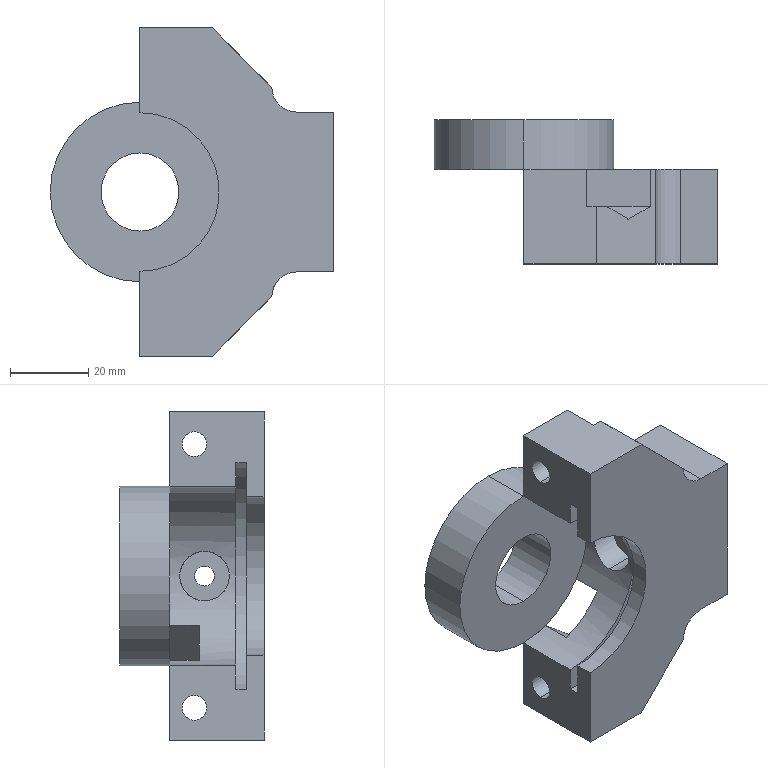Part | SolidWorks | features ICE 19, MirrorPattern 3, 3DProfileFeature 2, Fillet 2, RefAxis 2, Chamfer 1, CombineBodies 1, Cut 1, Extrusion 1, HoleWzd 1, MirrorSolid 1, MoveCopyBody 1, Stock 1 | 2 solids | 49 faces | box 72.644 x 36.906 x 84.074 mm | volume 68724 mm3 | plane 32 | cylinder 17 | commonest cylinder face diameters 6.35 x4 12.7 x4 45.974 x3 5.105 x2 20 x2 40.64 x1